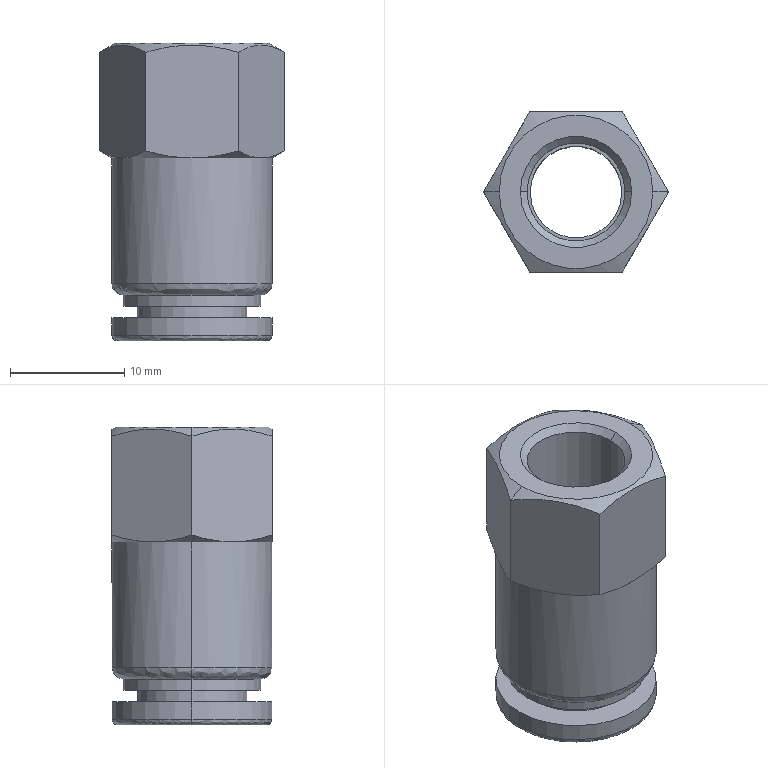Part | STEP file | APCF8-01 | 1 solid | 38 faces | box 16.166 x 14 x 26 mm | volume 2643 mm3 | cylinder 12 | cone 11 | plane 11 | spline 4 | commonest cylinder face diameters 14 x4 8 x2 8.566 x2 9.6 x2 12 x2
STEP:
#1=CARTESIAN_POINT('',(-7.,0.,5.));
#2=VERTEX_POINT('',#1);
#3=CARTESIAN_POINT('',(7.,0.,5.));
#4=VERTEX_POINT('',#3);
#5=CARTESIAN_POINT('',(0.,0.,5.));
#6=DIRECTION('',(0.,0.,1.));
#7=DIRECTION('',(-1.,0.,0.));
#8=AXIS2_PLACEMENT_3D('',#5,#6,#7);
#9=CIRCLE('',#8,7.);
#10=EDGE_CURVE('',#2,#4,#9,.T.);
#11=ORIENTED_EDGE('',*,*,#10,.F.);
#12=CARTESIAN_POINT('',(-6.,0.,4.));
#13=VERTEX_POINT('',#12);
#14=CARTESIAN_POINT('',(-6.,0.,5.));
#15=DIRECTION('',(0.,-1.,0.));
#16=DIRECTION('',(-1.,0.,0.));
#17=AXIS2_PLACEMENT_3D('',#14,#15,#16);
#18=CIRCLE('',#17,1.);
#19=EDGE_CURVE('',#2,#13,#18,.T.);
#20=ORIENTED_EDGE('',*,*,#19,.T.);
#21=CARTESIAN_POINT('',(6.,0.,4.));
#22=VERTEX_POINT('',#21);
#23=CARTESIAN_POINT('',(0.,0.,4.));
#24=DIRECTION('',(0.,0.,1.));
#25=DIRECTION('',(1.,0.,0.));
#26=AXIS2_PLACEMENT_3D('',#23,#24,#25);
#27=CIRCLE('',#26,6.);
#28=EDGE_CURVE('',#13,#22,#27,.T.);
#29=ORIENTED_EDGE('',*,*,#28,.T.);
#30=CARTESIAN_POINT('',(6.,0.,5.));
#31=DIRECTION('',(0.,1.,0.));
#32=DIRECTION('',(1.,0.,0.));
#33=AXIS2_PLACEMENT_3D('',#30,#31,#32);
#34=CIRCLE('',#33,1.);
#35=EDGE_CURVE('',#4,#22,#34,.T.);
#36=ORIENTED_EDGE('',*,*,#35,.F.);
#37=EDGE_LOOP('',(#11,#20,#29,#36));
#38=FACE_OUTER_BOUND('',#37,.T.);
#39=CARTESIAN_POINT('',(-7.,0.,5.));
#40=CARTESIAN_POINT('',(-7.,-14.,5.));
#41=CARTESIAN_POINT('',(7.,-14.,5.));
#42=CARTESIAN_POINT('',(7.,0.,5.));
#43=CARTESIAN_POINT('',(-7.,0.,4.414));
#44=CARTESIAN_POINT('',(-7.,-14.,4.414));
#45=CARTESIAN_POINT('',(7.,-14.,4.414));
#46=CARTESIAN_POINT('',(7.,0.,4.414));
#47=CARTESIAN_POINT('',(-6.586,0.,4.));
#48=CARTESIAN_POINT('',(-6.586,-13.172,4.));
#49=CARTESIAN_POINT('',(6.586,-13.172,4.));
#50=CARTESIAN_POINT('',(6.586,0.,4.));
#51=CARTESIAN_POINT('',(-6.,0.,4.));
#52=CARTESIAN_POINT('',(-6.,-12.,4.));
#53=CARTESIAN_POINT('',(6.,-12.,4.));
#54=CARTESIAN_POINT('',(6.,0.,4.));
#55=(BOUNDED_SURFACE()B_SPLINE_SURFACE(3,3,((#39,#40,#41,#42),(#43,#44,#45,#46),(#47,#48,#49,#50),(#51,#52,#53,#54)),.UNSPECIFIED.,.F.,.F.,.F.)B_SPLINE_SURFACE_WITH_KNOTS((4,4),(4,4),(0.,1.),(0.,1.),.UNSPECIFIED.)GEOMETRIC_REPRESENTATION_ITEM()RATIONAL_B_SPLINE_SURFACE(((1.,0.3333,0.3333,1.),(0.8047,0.2682,0.2682,0.8047),(0.8047,0.2682,0.2682,0.8047),(1.,0.3333,0.3333,1.)))REPRESENTATION_ITEM('')SURFACE());
#56=ADVANCED_FACE('',(#38),#55,.T.);
#57=CARTESIAN_POINT('',(-7.,0.,0.5));
#58=VERTEX_POINT('',#57);
#59=CARTESIAN_POINT('',(7.,0.,0.5));
#60=VERTEX_POINT('',#59);
#61=CARTESIAN_POINT('',(0.,0.,0.5));
#62=DIRECTION('',(0.,0.,1.));
#63=DIRECTION('',(-1.,0.,0.));
#64=AXIS2_PLACEMENT_3D('',#61,#62,#63);
#65=CIRCLE('',#64,7.);
#66=EDGE_CURVE('',#58,#60,#65,.T.);
#67=ORIENTED_EDGE('',*,*,#66,.F.);
#68=CARTESIAN_POINT('',(-6.5,0.,0.));
#69=VERTEX_POINT('',#68);
#70=CARTESIAN_POINT('',(-6.5,0.,0.5));
#71=DIRECTION('',(0.,-1.,0.));
#72=DIRECTION('',(-1.,0.,0.));
#73=AXIS2_PLACEMENT_3D('',#70,#71,#72);
#74=CIRCLE('',#73,0.5);
#75=EDGE_CURVE('',#58,#69,#74,.T.);
#76=ORIENTED_EDGE('',*,*,#75,.T.);
#77=CARTESIAN_POINT('',(6.5,0.,0.));
#78=VERTEX_POINT('',#77);
#79=CARTESIAN_POINT('',(-6.5,0.,0.));
#80=CARTESIAN_POINT('',(-6.5,-13.,0.));
#81=CARTESIAN_POINT('',(6.5,-13.,0.));
#82=CARTESIAN_POINT('',(6.5,0.,0.));
#83=(BOUNDED_CURVE()B_SPLINE_CURVE(3,(#79,#80,#81,#82),.UNSPECIFIED.,.F.,.T.)B_SPLINE_CURVE_WITH_KNOTS((4,4),(0.,1.),.UNSPECIFIED.)CURVE()GEOMETRIC_REPRESENTATION_ITEM()RATIONAL_B_SPLINE_CURVE((1.,0.3333,0.3333,1.))REPRESENTATION_ITEM(''));
#84=EDGE_CURVE('',#69,#78,#83,.T.);
#85=ORIENTED_EDGE('',*,*,#84,.T.);
#86=CARTESIAN_POINT('',(6.5,0.,0.5));
#87=DIRECTION('',(0.,1.,0.));
#88=DIRECTION('',(1.,0.,0.));
#89=AXIS2_PLACEMENT_3D('',#86,#87,#88);
#90=CIRCLE('',#89,0.5);
#91=EDGE_CURVE('',#60,#78,#90,.T.);
#92=ORIENTED_EDGE('',*,*,#91,.F.);
#93=EDGE_LOOP('',(#67,#76,#85,#92));
#94=FACE_OUTER_BOUND('',#93,.T.);
#95=CARTESIAN_POINT('',(-7.,0.,0.5));
#96=CARTESIAN_POINT('',(-7.,-14.,0.5));
#97=CARTESIAN_POINT('',(7.,-14.,0.5));
#98=CARTESIAN_POINT('',(7.,0.,0.5));
#99=CARTESIAN_POINT('',(-7.,0.,0.2071));
#100=CARTESIAN_POINT('',(-7.,-14.,0.2071));
#101=CARTESIAN_POINT('',(7.,-14.,0.2071));
#102=CARTESIAN_POINT('',(7.,0.,0.2071));
#103=CARTESIAN_POINT('',(-6.793,0.,0.));
#104=CARTESIAN_POINT('',(-6.793,-13.586,0.));
#105=CARTESIAN_POINT('',(6.793,-13.586,0.));
#106=CARTESIAN_POINT('',(6.793,0.,0.));
#107=CARTESIAN_POINT('',(-6.5,0.,0.));
#108=CARTESIAN_POINT('',(-6.5,-13.,0.));
#109=CARTESIAN_POINT('',(6.5,-13.,0.));
#110=CARTESIAN_POINT('',(6.5,0.,0.));
#111=(BOUNDED_SURFACE()B_SPLINE_SURFACE(3,3,((#95,#96,#97,#98),(#99,#100,#101,#102),(#103,#104,#105,#106),(#107,#108,#109,#110)),.UNSPECIFIED.,.F.,.F.,.F.)B_SPLINE_SURFACE_WITH_KNOTS((4,4),(4,4),(0.,1.),(0.,1.),.UNSPECIFIED.)GEOMETRIC_REPRESENTATION_ITEM()RATIONAL_B_SPLINE_SURFACE(((1.,0.3333,0.3333,1.),(0.8047,0.2682,0.2682,0.8047),(0.8047,0.2682,0.2682,0.8047),(1.,0.3333,0.3333,1.)))REPRESENTATION_ITEM('')SURFACE());
#112=ADVANCED_FACE('',(#94),#111,.T.);
#113=CARTESIAN_POINT('',(6.062,3.5,15.973));
#114=VERTEX_POINT('',#113);
#115=CARTESIAN_POINT('',(7.,0.,15.973));
#116=VERTEX_POINT('',#115);
#117=CARTESIAN_POINT('',(0.,0.,15.973));
#118=DIRECTION('',(0.,0.,-1.));
#119=DIRECTION('',(-1.,0.,0.));
#120=AXIS2_PLACEMENT_3D('',#117,#118,#119);
#121=CIRCLE('',#120,7.);
#122=EDGE_CURVE('',#114,#116,#121,.T.);
#123=ORIENTED_EDGE('',*,*,#122,.T.);
#124=CARTESIAN_POINT('',(7.,0.,10.487));
#125=DIRECTION('',(0.,0.,-1.));
#126=VECTOR('',#125,1000.);
#127=LINE('',#124,#126);
#128=EDGE_CURVE('',#116,#4,#127,.T.);
#129=ORIENTED_EDGE('',*,*,#128,.T.);
#130=CARTESIAN_POINT('',(0.,0.,5.));
#131=DIRECTION('',(0.,0.,1.));
#132=DIRECTION('',(-1.,0.,0.));
#133=AXIS2_PLACEMENT_3D('',#130,#131,#132);
#134=CIRCLE('',#133,7.);
#135=EDGE_CURVE('',#4,#2,#134,.T.);
#136=ORIENTED_EDGE('',*,*,#135,.T.);
#137=CARTESIAN_POINT('',(-7.,0.,15.973));
#138=VERTEX_POINT('',#137);
#139=CARTESIAN_POINT('',(-7.,0.,10.487));
#140=DIRECTION('',(0.,0.,-1.));
#141=VECTOR('',#140,1000.);
#142=LINE('',#139,#141);
#143=EDGE_CURVE('',#138,#2,#142,.T.);
#144=ORIENTED_EDGE('',*,*,#143,.F.);
#145=CARTESIAN_POINT('',(-6.062,3.5,15.973));
#146=VERTEX_POINT('',#145);
#147=CARTESIAN_POINT('',(0.,0.,15.973));
#148=DIRECTION('',(0.,0.,-1.));
#149=DIRECTION('',(-1.,0.,0.));
#150=AXIS2_PLACEMENT_3D('',#147,#148,#149);
#151=CIRCLE('',#150,7.);
#152=EDGE_CURVE('',#138,#146,#151,.T.);
#153=ORIENTED_EDGE('',*,*,#152,.T.);
#154=CARTESIAN_POINT('',(0.,7.,15.973));
#155=VERTEX_POINT('',#154);
#156=CARTESIAN_POINT('',(0.,0.,15.973));
#157=DIRECTION('',(0.,0.,-1.));
#158=DIRECTION('',(-1.,0.,0.));
#159=AXIS2_PLACEMENT_3D('',#156,#157,#158);
#160=CIRCLE('',#159,7.);
#161=EDGE_CURVE('',#146,#155,#160,.T.);
#162=ORIENTED_EDGE('',*,*,#161,.T.);
#163=CARTESIAN_POINT('',(0.,0.,15.973));
#164=DIRECTION('',(0.,0.,-1.));
#165=DIRECTION('',(-1.,0.,0.));
#166=AXIS2_PLACEMENT_3D('',#163,#164,#165);
#167=CIRCLE('',#166,7.);
#168=EDGE_CURVE('',#155,#114,#167,.T.);
#169=ORIENTED_EDGE('',*,*,#168,.T.);
#170=EDGE_LOOP('',(#123,#129,#136,#144,#153,#162,#169));
#171=FACE_OUTER_BOUND('',#170,.T.);
#172=CARTESIAN_POINT('',(0.,0.,10.487));
#173=DIRECTION('',(0.,0.,-1.));
#174=DIRECTION('',(-1.,0.,0.));
#175=AXIS2_PLACEMENT_3D('',#172,#173,#174);
#176=CYLINDRICAL_SURFACE('',#175,7.);
#177=ADVANCED_FACE('',(#171),#176,.T.);
#178=CARTESIAN_POINT('',(6.062,-3.5,15.973));
#179=VERTEX_POINT('',#178);
#180=CARTESIAN_POINT('',(0.,0.,15.973));
#181=DIRECTION('',(0.,0.,-1.));
#182=DIRECTION('',(-1.,0.,0.));
#183=AXIS2_PLACEMENT_3D('',#180,#181,#182);
#184=CIRCLE('',#183,7.);
#185=EDGE_CURVE('',#116,#179,#184,.T.);
#186=ORIENTED_EDGE('',*,*,#185,.F.);
#187=CARTESIAN_POINT('',(8.083,-0.000000012,16.598));
#188=VERTEX_POINT('',#187);
#189=CARTESIAN_POINT('',(8.089,0.,16.602));
#190=DIRECTION('',(0.866,0.,0.5));
#191=VECTOR('',#190,1000.);
#192=LINE('',#189,#191);
#193=EDGE_CURVE('',#116,#188,#192,.T.);
#194=ORIENTED_EDGE('',*,*,#193,.T.);
#195=CARTESIAN_POINT('',(8.083,-0.000000012,16.598));
#196=CARTESIAN_POINT('',(7.753,-0.5718,16.408));
#197=CARTESIAN_POINT('',(7.42,-1.148,16.251));
#198=CARTESIAN_POINT('',(6.747,-2.313,16.033));
#199=CARTESIAN_POINT('',(6.407,-2.903,15.973));
#200=CARTESIAN_POINT('',(6.062,-3.5,15.973));
#201=B_SPLINE_CURVE_WITH_KNOTS('',3,(#195,#196,#197,#198,#199,#200),.UNSPECIFIED.,.F.,.F.,(4,2,4),(0.,0.002045,0.00409),.UNSPECIFIED.);
#202=EDGE_CURVE('',#188,#179,#201,.T.);
#203=ORIENTED_EDGE('',*,*,#202,.T.);
#204=EDGE_LOOP('',(#186,#194,#203));
#205=FACE_OUTER_BOUND('',#204,.T.);
#206=CARTESIAN_POINT('',(0.,0.,16.602));
#207=DIRECTION('',(0.,0.,1.));
#208=DIRECTION('',(1.,0.,0.));
#209=AXIS2_PLACEMENT_3D('',#206,#207,#208);
#210=CONICAL_SURFACE('',#209,8.089,1.047);
#211=ADVANCED_FACE('',(#205),#210,.T.);
#212=CARTESIAN_POINT('',(0.,0.,4.));
#213=DIRECTION('',(0.,0.,1.));
#214=DIRECTION('',(1.,0.,0.));
#215=AXIS2_PLACEMENT_3D('',#212,#213,#214);
#216=CIRCLE('',#215,6.);
#217=EDGE_CURVE('',#22,#13,#216,.T.);
#218=ORIENTED_EDGE('',*,*,#217,.F.);
#219=CARTESIAN_POINT('',(6.,0.,3.));
#220=VERTEX_POINT('',#219);
#221=CARTESIAN_POINT('',(6.,0.,3.5));
#222=DIRECTION('',(0.,0.,-1.));
#223=VECTOR('',#222,1000.);
#224=LINE('',#221,#223);
#225=EDGE_CURVE('',#22,#220,#224,.T.);
#226=ORIENTED_EDGE('',*,*,#225,.T.);
#227=CARTESIAN_POINT('',(-6.,0.,3.));
#228=VERTEX_POINT('',#227);
#229=CARTESIAN_POINT('',(0.,0.,3.));
#230=DIRECTION('',(0.,0.,1.));
#231=DIRECTION('',(-1.,0.,0.));
#232=AXIS2_PLACEMENT_3D('',#229,#230,#231);
#233=CIRCLE('',#232,6.);
#234=EDGE_CURVE('',#220,#228,#233,.T.);
#235=ORIENTED_EDGE('',*,*,#234,.T.);
#236=CARTESIAN_POINT('',(-6.,0.,3.5));
#237=DIRECTION('',(0.,0.,-1.));
#238=VECTOR('',#237,1000.);
#239=LINE('',#236,#238);
#240=EDGE_CURVE('',#13,#228,#239,.T.);
#241=ORIENTED_EDGE('',*,*,#240,.F.);
#242=EDGE_LOOP('',(#218,#226,#235,#241));
#243=FACE_OUTER_BOUND('',#242,.T.);
#244=CARTESIAN_POINT('',(0.,0.,3.5));
#245=DIRECTION('',(0.,0.,-1.));
#246=DIRECTION('',(-1.,0.,0.));
#247=AXIS2_PLACEMENT_3D('',#244,#245,#246);
#248=CYLINDRICAL_SURFACE('',#247,6.);
#249=ADVANCED_FACE('',(#243),#248,.T.);
#250=CARTESIAN_POINT('',(-6.7,0.,26.));
#251=VERTEX_POINT('',#250);
#252=CARTESIAN_POINT('',(6.7,0.,26.));
#253=VERTEX_POINT('',#252);
#254=CARTESIAN_POINT('',(0.,0.,26.));
#255=DIRECTION('',(0.,0.,-1.));
#256=DIRECTION('',(-1.,0.,0.));
#257=AXIS2_PLACEMENT_3D('',#254,#255,#256);
#258=CIRCLE('',#257,6.7);
#259=EDGE_CURVE('',#251,#253,#258,.T.);
#260=ORIENTED_EDGE('',*,*,#259,.T.);
#261=CARTESIAN_POINT('',(8.083,0.,25.202));
#262=VERTEX_POINT('',#261);
#263=CARTESIAN_POINT('',(8.091,0.,25.197));
#264=DIRECTION('',(0.866,0.,-0.5));
#265=VECTOR('',#264,1000.);
#266=LINE('',#263,#265);
#267=EDGE_CURVE('',#253,#262,#266,.T.);
#268=ORIENTED_EDGE('',*,*,#267,.T.);
#269=CARTESIAN_POINT('',(4.041,7.,25.202));
#270=VERTEX_POINT('',#269);
#271=CARTESIAN_POINT('',(8.083,0.,25.202));
#272=CARTESIAN_POINT('',(7.753,0.5715,25.392));
#273=CARTESIAN_POINT('',(7.421,1.147,25.549));
#274=CARTESIAN_POINT('',(6.749,2.31,25.767));
#275=CARTESIAN_POINT('',(6.41,2.898,25.826));
#276=CARTESIAN_POINT('',(5.894,3.791,25.827));
#277=CARTESIAN_POINT('',(5.722,4.09,25.812));
#278=CARTESIAN_POINT('',(5.38,4.681,25.755));
#279=CARTESIAN_POINT('',(5.211,4.975,25.713));
#280=CARTESIAN_POINT('',(4.705,5.851,25.55));
#281=CARTESIAN_POINT('',(4.372,6.428,25.392));
#282=CARTESIAN_POINT('',(4.041,7.,25.202));
#283=B_SPLINE_CURVE_WITH_KNOTS('',3,(#271,#272,#273,#274,#275,#276,#277,#278,#279,#280,#281,#282),.UNSPECIFIED.,.F.,.F.,(4,2,2,2,2,4),(0.,0.002041,0.004082,0.005102,0.006122,0.008163),.UNSPECIFIED.);
#284=EDGE_CURVE('',#262,#270,#283,.T.);
#285=ORIENTED_EDGE('',*,*,#284,.T.);
#286=CARTESIAN_POINT('',(-4.041,7.,25.202));
#287=VERTEX_POINT('',#286);
#288=CARTESIAN_POINT('',(4.041,7.,25.202));
#289=CARTESIAN_POINT('',(3.381,7.,25.392));
#290=CARTESIAN_POINT('',(2.716,7.,25.549));
#291=CARTESIAN_POINT('',(1.37,7.,25.767));
#292=CARTESIAN_POINT('',(0.6897,7.,25.827));
#293=CARTESIAN_POINT('',(-0.6897,7.,25.827));
#294=CARTESIAN_POINT('',(-1.37,7.,25.767));
#295=CARTESIAN_POINT('',(-2.716,7.,25.549));
#296=CARTESIAN_POINT('',(-3.381,7.,25.392));
#297=CARTESIAN_POINT('',(-4.041,7.,25.202));
#298=B_SPLINE_CURVE_WITH_KNOTS('',3,(#288,#289,#290,#291,#292,#293,#294,#295,#296,#297),.UNSPECIFIED.,.F.,.F.,(4,2,2,2,4),(-0.00409,-0.002045,0.,0.002045,0.00409),.UNSPECIFIED.);
#299=EDGE_CURVE('',#270,#287,#298,.T.);
#300=ORIENTED_EDGE('',*,*,#299,.T.);
#301=CARTESIAN_POINT('',(-8.083,0.,25.202));
#302=VERTEX_POINT('',#301);
#303=CARTESIAN_POINT('',(-4.041,7.,25.202));
#304=CARTESIAN_POINT('',(-4.371,6.429,25.392));
#305=CARTESIAN_POINT('',(-4.704,5.853,25.549));
#306=CARTESIAN_POINT('',(-5.375,4.69,25.767));
#307=CARTESIAN_POINT('',(-5.715,4.102,25.826));
#308=CARTESIAN_POINT('',(-6.23,3.209,25.827));
#309=CARTESIAN_POINT('',(-6.403,2.91,25.812));
#310=CARTESIAN_POINT('',(-6.744,2.319,25.755));
#311=CARTESIAN_POINT('',(-6.914,2.025,25.713));
#312=CARTESIAN_POINT('',(-7.419,1.149,25.55));
#313=CARTESIAN_POINT('',(-7.753,0.5722,25.392));
#314=CARTESIAN_POINT('',(-8.083,0.,25.202));
#315=B_SPLINE_CURVE_WITH_KNOTS('',3,(#303,#304,#305,#306,#307,#308,#309,#310,#311,#312,#313,#314),.UNSPECIFIED.,.F.,.F.,(4,2,2,2,2,4),(0.,0.002041,0.004082,0.005102,0.006122,0.008163),.UNSPECIFIED.);
#316=EDGE_CURVE('',#287,#302,#315,.T.);
#317=ORIENTED_EDGE('',*,*,#316,.T.);
#318=CARTESIAN_POINT('',(-8.091,0.,25.197));
#319=DIRECTION('',(-0.866,0.,-0.5));
#320=VECTOR('',#319,1000.);
#321=LINE('',#318,#320);
#322=EDGE_CURVE('',#251,#302,#321,.T.);
#323=ORIENTED_EDGE('',*,*,#322,.F.);
#324=EDGE_LOOP('',(#260,#268,#285,#300,#317,#323));
#325=FACE_OUTER_BOUND('',#324,.T.);
#326=CARTESIAN_POINT('',(0.,0.,25.197));
#327=DIRECTION('',(0.,0.,-1.));
#328=DIRECTION('',(-1.,0.,0.));
#329=AXIS2_PLACEMENT_3D('',#326,#327,#328);
#330=CONICAL_SURFACE('',#329,8.091,1.047);
#331=ADVANCED_FACE('',(#325),#330,.T.);
#332=CARTESIAN_POINT('',(4.8,0.,3.));
#333=VERTEX_POINT('',#332);
#334=CARTESIAN_POINT('',(-4.8,0.,3.));
#335=VERTEX_POINT('',#334);
#336=CARTESIAN_POINT('',(0.,0.,3.));
#337=DIRECTION('',(0.,0.,1.));
#338=DIRECTION('',(-1.,0.,0.));
#339=AXIS2_PLACEMENT_3D('',#336,#337,#338);
#340=CIRCLE('',#339,4.8);
#341=EDGE_CURVE('',#333,#335,#340,.T.);
#342=ORIENTED_EDGE('',*,*,#341,.F.);
#343=CARTESIAN_POINT('',(4.8,0.,2.));
#344=VERTEX_POINT('',#343);
#345=CARTESIAN_POINT('',(4.8,0.,2.5));
#346=DIRECTION('',(0.,0.,-1.));
#347=VECTOR('',#346,1000.);
#348=LINE('',#345,#347);
#349=EDGE_CURVE('',#333,#344,#348,.T.);
#350=ORIENTED_EDGE('',*,*,#349,.T.);
#351=CARTESIAN_POINT('',(-4.8,0.,2.));
#352=VERTEX_POINT('',#351);
#353=CARTESIAN_POINT('',(0.,0.,2.));
#354=DIRECTION('',(0.,0.,1.));
#355=DIRECTION('',(-1.,0.,0.));
#356=AXIS2_PLACEMENT_3D('',#353,#354,#355);
#357=CIRCLE('',#356,4.8);
#358=EDGE_CURVE('',#344,#352,#357,.T.);
#359=ORIENTED_EDGE('',*,*,#358,.T.);
#360=CARTESIAN_POINT('',(-4.8,0.,2.5));
#361=DIRECTION('',(0.,0.,-1.));
#362=VECTOR('',#361,1000.);
#363=LINE('',#360,#362);
#364=EDGE_CURVE('',#335,#352,#363,.T.);
#365=ORIENTED_EDGE('',*,*,#364,.F.);
#366=EDGE_LOOP('',(#342,#350,#359,#365));
#367=FACE_OUTER_BOUND('',#366,.T.);
#368=CARTESIAN_POINT('',(0.,0.,2.5));
#369=DIRECTION('',(0.,0.,-1.));
#370=DIRECTION('',(-1.,0.,0.));
#371=AXIS2_PLACEMENT_3D('',#368,#369,#370);
#372=CYLINDRICAL_SURFACE('',#371,4.8);
#373=ADVANCED_FACE('',(#367),#372,.T.);
#374=CARTESIAN_POINT('',(-4.283,0.,25.419));
#375=VERTEX_POINT('',#374);
#376=CARTESIAN_POINT('',(4.283,0.,25.419));
#377=VERTEX_POINT('',#376);
#378=CARTESIAN_POINT('',(0.,0.,25.419));
#379=DIRECTION('',(0.,0.,1.));
#380=DIRECTION('',(0.,1.,0.));
#381=AXIS2_PLACEMENT_3D('',#378,#379,#380);
#382=CIRCLE('',#381,4.283);
#383=EDGE_CURVE('',#375,#377,#382,.T.);
#384=ORIENTED_EDGE('',*,*,#383,.F.);
#385=CARTESIAN_POINT('',(-4.864,0.,26.));
#386=VERTEX_POINT('',#385);
#387=CARTESIAN_POINT('',(-4.864,0.,26.));
#388=DIRECTION('',(-0.7071,0.,0.7071));
#389=VECTOR('',#388,1000.);
#390=LINE('',#387,#389);
#391=EDGE_CURVE('',#375,#386,#390,.T.);
#392=ORIENTED_EDGE('',*,*,#391,.T.);
#393=CARTESIAN_POINT('',(4.864,0.,26.));
#394=VERTEX_POINT('',#393);
#395=CARTESIAN_POINT('',(0.,0.,26.));
#396=DIRECTION('',(0.,0.,-1.));
#397=DIRECTION('',(1.,0.,0.));
#398=AXIS2_PLACEMENT_3D('',#395,#396,#397);
#399=CIRCLE('',#398,4.864);
#400=EDGE_CURVE('',#394,#386,#399,.T.);
#401=ORIENTED_EDGE('',*,*,#400,.F.);
#402=CARTESIAN_POINT('',(4.864,0.,26.));
#403=DIRECTION('',(0.7071,0.,0.7071));
#404=VECTOR('',#403,1000.);
#405=LINE('',#402,#404);
#406=EDGE_CURVE('',#377,#394,#405,.T.);
#407=ORIENTED_EDGE('',*,*,#406,.F.);
#408=EDGE_LOOP('',(#384,#392,#401,#407));
#409=FACE_OUTER_BOUND('',#408,.T.);
#410=CARTESIAN_POINT('',(0.,0.,26.));
#411=DIRECTION('',(0.,0.,1.));
#412=DIRECTION('',(1.,0.,0.));
#413=AXIS2_PLACEMENT_3D('',#410,#411,#412);
#414=CONICAL_SURFACE('',#413,4.864,0.7854);
#415=ADVANCED_FACE('',(#409),#414,.F.);
#416=CARTESIAN_POINT('',(7.,0.,2.));
#417=VERTEX_POINT('',#416);
#418=CARTESIAN_POINT('',(-7.,0.,2.));
#419=VERTEX_POINT('',#418);
#420=CARTESIAN_POINT('',(0.,0.,2.));
#421=DIRECTION('',(0.,0.,1.));
#422=DIRECTION('',(-1.,0.,0.));
#423=AXIS2_PLACEMENT_3D('',#420,#421,#422);
#424=CIRCLE('',#423,7.);
#425=EDGE_CURVE('',#417,#419,#424,.T.);
#426=ORIENTED_EDGE('',*,*,#425,.F.);
#427=CARTESIAN_POINT('',(7.,0.,1.25));
#428=DIRECTION('',(0.,0.,-1.));
#429=VECTOR('',#428,1000.);
#430=LINE('',#427,#429);
#431=EDGE_CURVE('',#417,#60,#430,.T.);
#432=ORIENTED_EDGE('',*,*,#431,.T.);
#433=CARTESIAN_POINT('',(0.,0.,0.5));
#434=DIRECTION('',(0.,0.,1.));
#435=DIRECTION('',(-1.,0.,0.));
#436=AXIS2_PLACEMENT_3D('',#433,#434,#435);
#437=CIRCLE('',#436,7.);
#438=EDGE_CURVE('',#60,#58,#437,.T.);
#439=ORIENTED_EDGE('',*,*,#438,.T.);
#440=CARTESIAN_POINT('',(-7.,0.,1.25));
#441=DIRECTION('',(0.,0.,-1.));
#442=VECTOR('',#441,1000.);
#443=LINE('',#440,#442);
#444=EDGE_CURVE('',#419,#58,#443,.T.);
#445=ORIENTED_EDGE('',*,*,#444,.F.);
#446=EDGE_LOOP('',(#426,#432,#439,#445));
#447=FACE_OUTER_BOUND('',#446,.T.);
#448=CARTESIAN_POINT('',(0.,0.,1.25));
#449=DIRECTION('',(0.,0.,-1.));
#450=DIRECTION('',(-1.,0.,0.));
#451=AXIS2_PLACEMENT_3D('',#448,#449,#450);
#452=CYLINDRICAL_SURFACE('',#451,7.);
#453=ADVANCED_FACE('',(#447),#452,.T.);
#454=ORIENTED_EDGE('',*,*,#383,.T.);
#455=CARTESIAN_POINT('',(4.283,0.,17.5));
#456=VERTEX_POINT('',#455);
#457=CARTESIAN_POINT('',(4.283,0.,21.459));
#458=DIRECTION('',(0.,0.,-1.));
#459=VECTOR('',#458,1000.);
#460=LINE('',#457,#459);
#461=EDGE_CURVE('',#377,#456,#460,.T.);
#462=ORIENTED_EDGE('',*,*,#461,.T.);
#463=CARTESIAN_POINT('',(-4.283,0.,17.5));
#464=VERTEX_POINT('',#463);
#465=CARTESIAN_POINT('',(0.,0.,17.5));
#466=DIRECTION('',(0.,0.,1.));
#467=DIRECTION('',(-1.,0.,0.));
#468=AXIS2_PLACEMENT_3D('',#465,#466,#467);
#469=CIRCLE('',#468,4.283);
#470=EDGE_CURVE('',#464,#456,#469,.T.);
#471=ORIENTED_EDGE('',*,*,#470,.F.);
#472=CARTESIAN_POINT('',(-4.283,0.,21.459));
#473=DIRECTION('',(0.,0.,-1.));
#474=VECTOR('',#473,1000.);
#475=LINE('',#472,#474);
#476=EDGE_CURVE('',#375,#464,#475,.T.);
#477=ORIENTED_EDGE('',*,*,#476,.F.);
#478=EDGE_LOOP('',(#454,#462,#471,#477));
#479=FACE_OUTER_BOUND('',#478,.T.);
#480=CARTESIAN_POINT('',(0.,0.,21.459));
#481=DIRECTION('',(0.,0.,-1.));
#482=DIRECTION('',(-1.,0.,0.));
#483=AXIS2_PLACEMENT_3D('',#480,#481,#482);
#484=CYLINDRICAL_SURFACE('',#483,4.283);
#485=ADVANCED_FACE('',(#479),#484,.F.);
#486=CARTESIAN_POINT('',(4.,0.,17.5));
#487=VERTEX_POINT('',#486);
#488=CARTESIAN_POINT('',(-4.,0.,17.5));
#489=VERTEX_POINT('',#488);
#490=CARTESIAN_POINT('',(0.,0.,17.5));
#491=DIRECTION('',(0.,0.,-1.));
#492=DIRECTION('',(-1.,0.,0.));
#493=AXIS2_PLACEMENT_3D('',#490,#491,#492);
#494=CIRCLE('',#493,4.);
#495=EDGE_CURVE('',#487,#489,#494,.T.);
#496=ORIENTED_EDGE('',*,*,#495,.F.);
#497=CARTESIAN_POINT('',(4.,0.,0.));
#498=VERTEX_POINT('',#497);
#499=CARTESIAN_POINT('',(4.,0.,8.75));
#500=DIRECTION('',(0.,0.,-1.));
#501=VECTOR('',#500,1000.);
#502=LINE('',#499,#501);
#503=EDGE_CURVE('',#487,#498,#502,.T.);
#504=ORIENTED_EDGE('',*,*,#503,.T.);
#505=CARTESIAN_POINT('',(-4.,0.,0.));
#506=VERTEX_POINT('',#505);
#507=CARTESIAN_POINT('',(0.,0.,0.));
#508=DIRECTION('',(0.,0.,1.));
#509=DIRECTION('',(-1.,0.,0.));
#510=AXIS2_PLACEMENT_3D('',#507,#508,#509);
#511=CIRCLE('',#510,4.);
#512=EDGE_CURVE('',#506,#498,#511,.T.);
#513=ORIENTED_EDGE('',*,*,#512,.F.);
#514=CARTESIAN_POINT('',(-4.,0.,8.75));
#515=DIRECTION('',(0.,0.,-1.));
#516=VECTOR('',#515,1000.);
#517=LINE('',#514,#516);
#518=EDGE_CURVE('',#489,#506,#517,.T.);
#519=ORIENTED_EDGE('',*,*,#518,.F.);
#520=EDGE_LOOP('',(#496,#504,#513,#519));
#521=FACE_OUTER_BOUND('',#520,.T.);
#522=CARTESIAN_POINT('',(0.,0.,8.75));
#523=DIRECTION('',(0.,0.,-1.));
#524=DIRECTION('',(-1.,0.,0.));
#525=AXIS2_PLACEMENT_3D('',#522,#523,#524);
#526=CYLINDRICAL_SURFACE('',#525,4.);
#527=ADVANCED_FACE('',(#521),#526,.F.);
#528=ORIENTED_EDGE('',*,*,#128,.F.);
#529=ORIENTED_EDGE('',*,*,#185,.T.);
#530=CARTESIAN_POINT('',(0.,-7.,15.973));
#531=VERTEX_POINT('',#530);
#532=CARTESIAN_POINT('',(0.,0.,15.973));
#533=DIRECTION('',(0.,0.,-1.));
#534=DIRECTION('',(-1.,0.,0.));
#535=AXIS2_PLACEMENT_3D('',#532,#533,#534);
#536=CIRCLE('',#535,7.);
#537=EDGE_CURVE('',#179,#531,#536,.T.);
#538=ORIENTED_EDGE('',*,*,#537,.T.);
#539=CARTESIAN_POINT('',(-6.062,-3.5,15.973));
#540=VERTEX_POINT('',#539);
#541=CARTESIAN_POINT('',(0.,0.,15.973));
#542=DIRECTION('',(0.,0.,-1.));
#543=DIRECTION('',(-1.,0.,0.));
#544=AXIS2_PLACEMENT_3D('',#541,#542,#543);
#545=CIRCLE('',#544,7.);
#546=EDGE_CURVE('',#531,#540,#545,.T.);
#547=ORIENTED_EDGE('',*,*,#546,.T.);
#548=CARTESIAN_POINT('',(0.,0.,15.973));
#549=DIRECTION('',(0.,0.,-1.));
#550=DIRECTION('',(-1.,0.,0.));
#551=AXIS2_PLACEMENT_3D('',#548,#549,#550);
#552=CIRCLE('',#551,7.);
#553=EDGE_CURVE('',#540,#138,#552,.T.);
#554=ORIENTED_EDGE('',*,*,#553,.T.);
#555=ORIENTED_EDGE('',*,*,#143,.T.);
#556=ORIENTED_EDGE('',*,*,#10,.T.);
#557=EDGE_LOOP('',(#528,#529,#538,#547,#554,#555,#556));
#558=FACE_OUTER_BOUND('',#557,.T.);
#559=CARTESIAN_POINT('',(0.,0.,10.487));
#560=DIRECTION('',(0.,0.,-1.));
#561=DIRECTION('',(-1.,0.,0.));
#562=AXIS2_PLACEMENT_3D('',#559,#560,#561);
#563=CYLINDRICAL_SURFACE('',#562,7.);
#564=ADVANCED_FACE('',(#558),#563,.T.);
#565=ORIENTED_EDGE('',*,*,#19,.F.);
#566=ORIENTED_EDGE('',*,*,#135,.F.);
#567=ORIENTED_EDGE('',*,*,#35,.T.);
#568=ORIENTED_EDGE('',*,*,#217,.T.);
#569=EDGE_LOOP('',(#565,#566,#567,#568));
#570=FACE_OUTER_BOUND('',#569,.T.);
#571=CARTESIAN_POINT('',(7.,0.,5.));
#572=CARTESIAN_POINT('',(7.,14.,5.));
#573=CARTESIAN_POINT('',(-7.,14.,5.));
#574=CARTESIAN_POINT('',(-7.,0.,5.));
#575=CARTESIAN_POINT('',(7.,0.,4.414));
#576=CARTESIAN_POINT('',(7.,14.,4.414));
#577=CARTESIAN_POINT('',(-7.,14.,4.414));
#578=CARTESIAN_POINT('',(-7.,0.,4.414));
#579=CARTESIAN_POINT('',(6.586,0.,4.));
#580=CARTESIAN_POINT('',(6.586,13.172,4.));
#581=CARTESIAN_POINT('',(-6.586,13.172,4.));
#582=CARTESIAN_POINT('',(-6.586,0.,4.));
#583=CARTESIAN_POINT('',(6.,0.,4.));
#584=CARTESIAN_POINT('',(6.,12.,4.));
#585=CARTESIAN_POINT('',(-6.,12.,4.));
#586=CARTESIAN_POINT('',(-6.,0.,4.));
#587=(BOUNDED_SURFACE()B_SPLINE_SURFACE(3,3,((#571,#572,#573,#574),(#575,#576,#577,#578),(#579,#580,#581,#582),(#583,#584,#585,#586)),.UNSPECIFIED.,.F.,.F.,.F.)B_SPLINE_SURFACE_WITH_KNOTS((4,4),(4,4),(0.,1.),(0.,1.),.UNSPECIFIED.)GEOMETRIC_REPRESENTATION_ITEM()RATIONAL_B_SPLINE_SURFACE(((1.,0.3333,0.3333,1.),(0.8047,0.2682,0.2682,0.8047),(0.8047,0.2682,0.2682,0.8047),(1.,0.3333,0.3333,1.)))REPRESENTATION_ITEM('')SURFACE());
#588=ADVANCED_FACE('',(#570),#587,.T.);
#589=CARTESIAN_POINT('',(4.041,-7.,16.598));
#590=VERTEX_POINT('',#589);
#591=CARTESIAN_POINT('',(4.041,-7.,16.598));
#592=CARTESIAN_POINT('',(3.381,-7.,16.408));
#593=CARTESIAN_POINT('',(2.716,-7.,16.251));
#594=CARTESIAN_POINT('',(1.37,-7.,16.033));
#595=CARTESIAN_POINT('',(0.6897,-7.,15.973));
#596=CARTESIAN_POINT('',(0.,-7.,15.973));
#597=B_SPLINE_CURVE_WITH_KNOTS('',3,(#591,#592,#593,#594,#595,#596),.UNSPECIFIED.,.F.,.F.,(4,2,4),(0.,0.002045,0.00409),.UNSPECIFIED.);
#598=EDGE_CURVE('',#590,#531,#597,.T.);
#599=ORIENTED_EDGE('',*,*,#598,.T.);
#600=ORIENTED_EDGE('',*,*,#537,.F.);
#601=CARTESIAN_POINT('',(6.062,-3.5,15.973));
#602=CARTESIAN_POINT('',(5.717,-4.097,15.973));
#603=CARTESIAN_POINT('',(5.377,-4.687,16.033));
#604=CARTESIAN_POINT('',(4.704,-5.852,16.251));
#605=CARTESIAN_POINT('',(4.372,-6.428,16.408));
#606=CARTESIAN_POINT('',(4.041,-7.,16.598));
#607=B_SPLINE_CURVE_WITH_KNOTS('',3,(#601,#602,#603,#604,#605,#606),.UNSPECIFIED.,.F.,.F.,(4,2,4),(0.,0.002045,0.00409),.UNSPECIFIED.);
#608=EDGE_CURVE('',#179,#590,#607,.T.);
#609=ORIENTED_EDGE('',*,*,#608,.T.);
#610=EDGE_LOOP('',(#599,#600,#609));
#611=FACE_OUTER_BOUND('',#610,.T.);
#612=CARTESIAN_POINT('',(0.,0.,16.602));
#613=DIRECTION('',(0.,0.,1.));
#614=DIRECTION('',(1.,0.,0.));
#615=AXIS2_PLACEMENT_3D('',#612,#613,#614);
#616=CONICAL_SURFACE('',#615,8.089,1.047);
#617=ADVANCED_FACE('',(#611),#616,.T.);
#618=ORIENTED_EDGE('',*,*,#193,.F.);
#619=ORIENTED_EDGE('',*,*,#122,.F.);
#620=CARTESIAN_POINT('',(6.062,3.5,15.973));
#621=CARTESIAN_POINT('',(6.407,2.903,15.973));
#622=CARTESIAN_POINT('',(6.747,2.313,16.033));
#623=CARTESIAN_POINT('',(7.42,1.148,16.251));
#624=CARTESIAN_POINT('',(7.753,0.5718,16.408));
#625=CARTESIAN_POINT('',(8.083,-0.000000012,16.598));
#626=B_SPLINE_CURVE_WITH_KNOTS('',3,(#620,#621,#622,#623,#624,#625),.UNSPECIFIED.,.F.,.F.,(4,2,4),(0.,0.002045,0.00409),.UNSPECIFIED.);
#627=EDGE_CURVE('',#114,#188,#626,.T.);
#628=ORIENTED_EDGE('',*,*,#627,.T.);
#629=EDGE_LOOP('',(#618,#619,#628));
#630=FACE_OUTER_BOUND('',#629,.T.);
#631=CARTESIAN_POINT('',(0.,0.,16.602));
#632=DIRECTION('',(0.,0.,1.));
#633=DIRECTION('',(1.,0.,0.));
#634=AXIS2_PLACEMENT_3D('',#631,#632,#633);
#635=CONICAL_SURFACE('',#634,8.089,1.047);
#636=ADVANCED_FACE('',(#630),#635,.T.);
#637=ORIENTED_EDGE('',*,*,#168,.F.);
#638=CARTESIAN_POINT('',(4.041,7.,16.598));
#639=VERTEX_POINT('',#638);
#640=CARTESIAN_POINT('',(0.,7.,15.973));
#641=CARTESIAN_POINT('',(0.6897,7.,15.973));
#642=CARTESIAN_POINT('',(1.37,7.,16.033));
#643=CARTESIAN_POINT('',(2.716,7.,16.251));
#644=CARTESIAN_POINT('',(3.381,7.,16.408));
#645=CARTESIAN_POINT('',(4.041,7.,16.598));
#646=B_SPLINE_CURVE_WITH_KNOTS('',3,(#640,#641,#642,#643,#644,#645),.UNSPECIFIED.,.F.,.F.,(4,2,4),(0.,0.002045,0.00409),.UNSPECIFIED.);
#647=EDGE_CURVE('',#155,#639,#646,.T.);
#648=ORIENTED_EDGE('',*,*,#647,.T.);
#649=CARTESIAN_POINT('',(4.041,7.,16.598));
#650=CARTESIAN_POINT('',(4.372,6.428,16.408));
#651=CARTESIAN_POINT('',(4.704,5.852,16.251));
#652=CARTESIAN_POINT('',(5.377,4.687,16.033));
#653=CARTESIAN_POINT('',(5.717,4.097,15.973));
#654=CARTESIAN_POINT('',(6.062,3.5,15.973));
#655=B_SPLINE_CURVE_WITH_KNOTS('',3,(#649,#650,#651,#652,#653,#654),.UNSPECIFIED.,.F.,.F.,(4,2,4),(0.,0.002045,0.00409),.UNSPECIFIED.);
#656=EDGE_CURVE('',#639,#114,#655,.T.);
#657=ORIENTED_EDGE('',*,*,#656,.T.);
#658=EDGE_LOOP('',(#637,#648,#657));
#659=FACE_OUTER_BOUND('',#658,.T.);
#660=CARTESIAN_POINT('',(0.,0.,16.602));
#661=DIRECTION('',(0.,0.,1.));
#662=DIRECTION('',(1.,0.,0.));
#663=AXIS2_PLACEMENT_3D('',#660,#661,#662);
#664=CONICAL_SURFACE('',#663,8.089,1.047);
#665=ADVANCED_FACE('',(#659),#664,.T.);
#666=ORIENTED_EDGE('',*,*,#225,.F.);
#667=ORIENTED_EDGE('',*,*,#28,.F.);
#668=ORIENTED_EDGE('',*,*,#240,.T.);
#669=CARTESIAN_POINT('',(0.,0.,3.));
#670=DIRECTION('',(0.,0.,1.));
#671=DIRECTION('',(-1.,0.,0.));
#672=AXIS2_PLACEMENT_3D('',#669,#670,#671);
#673=CIRCLE('',#672,6.);
#674=EDGE_CURVE('',#228,#220,#673,.T.);
#675=ORIENTED_EDGE('',*,*,#674,.T.);
#676=EDGE_LOOP('',(#666,#667,#668,#675));
#677=FACE_OUTER_BOUND('',#676,.T.);
#678=CARTESIAN_POINT('',(0.,0.,3.5));
#679=DIRECTION('',(0.,0.,-1.));
#680=DIRECTION('',(-1.,0.,0.));
#681=AXIS2_PLACEMENT_3D('',#678,#679,#680);
#682=CYLINDRICAL_SURFACE('',#681,6.);
#683=ADVANCED_FACE('',(#677),#682,.T.);
#684=ORIENTED_EDGE('',*,*,#161,.F.);
#685=CARTESIAN_POINT('',(-4.041,7.,16.598));
#686=VERTEX_POINT('',#685);
#687=CARTESIAN_POINT('',(-6.062,3.5,15.973));
#688=CARTESIAN_POINT('',(-5.717,4.097,15.973));
#689=CARTESIAN_POINT('',(-5.377,4.687,16.033));
#690=CARTESIAN_POINT('',(-4.704,5.852,16.251));
#691=CARTESIAN_POINT('',(-4.372,6.428,16.408));
#692=CARTESIAN_POINT('',(-4.041,7.,16.598));
#693=B_SPLINE_CURVE_WITH_KNOTS('',3,(#687,#688,#689,#690,#691,#692),.UNSPECIFIED.,.F.,.F.,(4,2,4),(0.,0.002045,0.00409),.UNSPECIFIED.);
#694=EDGE_CURVE('',#146,#686,#693,.T.);
#695=ORIENTED_EDGE('',*,*,#694,.T.);
#696=CARTESIAN_POINT('',(-4.041,7.,16.598));
#697=CARTESIAN_POINT('',(-3.381,7.,16.408));
#698=CARTESIAN_POINT('',(-2.716,7.,16.251));
#699=CARTESIAN_POINT('',(-1.37,7.,16.033));
#700=CARTESIAN_POINT('',(-0.6897,7.,15.973));
#701=CARTESIAN_POINT('',(0.,7.,15.973));
#702=B_SPLINE_CURVE_WITH_KNOTS('',3,(#696,#697,#698,#699,#700,#701),.UNSPECIFIED.,.F.,.F.,(4,2,4),(0.,0.002045,0.00409),.UNSPECIFIED.);
#703=EDGE_CURVE('',#686,#155,#702,.T.);
#704=ORIENTED_EDGE('',*,*,#703,.T.);
#705=EDGE_LOOP('',(#684,#695,#704));
#706=FACE_OUTER_BOUND('',#705,.T.);
#707=CARTESIAN_POINT('',(0.,0.,16.602));
#708=DIRECTION('',(0.,0.,1.));
#709=DIRECTION('',(1.,0.,0.));
#710=AXIS2_PLACEMENT_3D('',#707,#708,#709);
#711=CONICAL_SURFACE('',#710,8.089,1.047);
#712=ADVANCED_FACE('',(#706),#711,.T.);
#713=ORIENTED_EDGE('',*,*,#553,.F.);
#714=CARTESIAN_POINT('',(-8.083,0.000000038,16.598));
#715=VERTEX_POINT('',#714);
#716=CARTESIAN_POINT('',(-6.062,-3.5,15.973));
#717=CARTESIAN_POINT('',(-6.407,-2.903,15.973));
#718=CARTESIAN_POINT('',(-6.747,-2.313,16.033));
#719=CARTESIAN_POINT('',(-7.42,-1.148,16.251));
#720=CARTESIAN_POINT('',(-7.753,-0.5718,16.408));
#721=CARTESIAN_POINT('',(-8.083,0.000000038,16.598));
#722=B_SPLINE_CURVE_WITH_KNOTS('',3,(#716,#717,#718,#719,#720,#721),.UNSPECIFIED.,.F.,.F.,(4,2,4),(0.,0.002045,0.00409),.UNSPECIFIED.);
#723=EDGE_CURVE('',#540,#715,#722,.T.);
#724=ORIENTED_EDGE('',*,*,#723,.T.);
#725=CARTESIAN_POINT('',(-8.083,0.000000038,16.598));
#726=CARTESIAN_POINT('',(-7.753,0.5718,16.408));
#727=CARTESIAN_POINT('',(-7.42,1.148,16.251));
#728=CARTESIAN_POINT('',(-6.747,2.313,16.033));
#729=CARTESIAN_POINT('',(-6.407,2.903,15.973));
#730=CARTESIAN_POINT('',(-6.062,3.5,15.973));
#731=B_SPLINE_CURVE_WITH_KNOTS('',3,(#725,#726,#727,#728,#729,#730),.UNSPECIFIED.,.F.,.F.,(4,2,4),(0.,0.002045,0.00409),.UNSPECIFIED.);
#732=EDGE_CURVE('',#715,#146,#731,.T.);
#733=ORIENTED_EDGE('',*,*,#732,.T.);
#734=ORIENTED_EDGE('',*,*,#152,.F.);
#735=EDGE_LOOP('',(#713,#724,#733,#734));
#736=FACE_OUTER_BOUND('',#735,.T.);
#737=CARTESIAN_POINT('',(0.,0.,16.602));
#738=DIRECTION('',(0.,0.,1.));
#739=DIRECTION('',(1.,0.,0.));
#740=AXIS2_PLACEMENT_3D('',#737,#738,#739);
#741=CONICAL_SURFACE('',#740,8.089,1.047);
#742=ADVANCED_FACE('',(#736),#741,.T.);
#743=CARTESIAN_POINT('',(-4.041,-7.,16.598));
#744=VERTEX_POINT('',#743);
#745=CARTESIAN_POINT('',(-4.041,-7.,16.598));
#746=CARTESIAN_POINT('',(-4.372,-6.428,16.408));
#747=CARTESIAN_POINT('',(-4.704,-5.852,16.251));
#748=CARTESIAN_POINT('',(-5.377,-4.687,16.033));
#749=CARTESIAN_POINT('',(-5.717,-4.097,15.973));
#750=CARTESIAN_POINT('',(-6.062,-3.5,15.973));
#751=B_SPLINE_CURVE_WITH_KNOTS('',3,(#745,#746,#747,#748,#749,#750),.UNSPECIFIED.,.F.,.F.,(4,2,4),(0.,0.002045,0.00409),.UNSPECIFIED.);
#752=EDGE_CURVE('',#744,#540,#751,.T.);
#753=ORIENTED_EDGE('',*,*,#752,.T.);
#754=ORIENTED_EDGE('',*,*,#546,.F.);
#755=CARTESIAN_POINT('',(0.,-7.,15.973));
#756=CARTESIAN_POINT('',(-0.6897,-7.,15.973));
#757=CARTESIAN_POINT('',(-1.37,-7.,16.033));
#758=CARTESIAN_POINT('',(-2.716,-7.,16.251));
#759=CARTESIAN_POINT('',(-3.381,-7.,16.408));
#760=CARTESIAN_POINT('',(-4.041,-7.,16.598));
#761=B_SPLINE_CURVE_WITH_KNOTS('',3,(#755,#756,#757,#758,#759,#760),.UNSPECIFIED.,.F.,.F.,(4,2,4),(0.,0.002045,0.00409),.UNSPECIFIED.);
#762=EDGE_CURVE('',#531,#744,#761,.T.);
#763=ORIENTED_EDGE('',*,*,#762,.T.);
#764=EDGE_LOOP('',(#753,#754,#763));
#765=FACE_OUTER_BOUND('',#764,.T.);
#766=CARTESIAN_POINT('',(0.,0.,16.602));
#767=DIRECTION('',(0.,0.,1.));
#768=DIRECTION('',(1.,0.,0.));
#769=AXIS2_PLACEMENT_3D('',#766,#767,#768);
#770=CONICAL_SURFACE('',#769,8.089,1.047);
#771=ADVANCED_FACE('',(#765),#770,.T.);
#772=CARTESIAN_POINT('',(-4.041,-7.,25.202));
#773=VERTEX_POINT('',#772);
#774=CARTESIAN_POINT('',(-4.041,-7.,26.));
#775=DIRECTION('',(0.,0.,1.));
#776=VECTOR('',#775,1000.);
#777=LINE('',#774,#776);
#778=EDGE_CURVE('',#744,#773,#777,.T.);
#779=ORIENTED_EDGE('',*,*,#778,.F.);
#780=ORIENTED_EDGE('',*,*,#762,.F.);
#781=ORIENTED_EDGE('',*,*,#598,.F.);
#782=CARTESIAN_POINT('',(4.041,-7.,25.202));
#783=VERTEX_POINT('',#782);
#784=CARTESIAN_POINT('',(4.041,-7.,26.));
#785=DIRECTION('',(0.,0.,-1.));
#786=VECTOR('',#785,1000.);
#787=LINE('',#784,#786);
#788=EDGE_CURVE('',#783,#590,#787,.T.);
#789=ORIENTED_EDGE('',*,*,#788,.F.);
#790=CARTESIAN_POINT('',(-4.041,-7.,25.202));
#791=CARTESIAN_POINT('',(-3.381,-7.,25.392));
#792=CARTESIAN_POINT('',(-2.716,-7.,25.549));
#793=CARTESIAN_POINT('',(-1.37,-7.,25.767));
#794=CARTESIAN_POINT('',(-0.6897,-7.,25.827));
#795=CARTESIAN_POINT('',(0.6897,-7.,25.827));
#796=CARTESIAN_POINT('',(1.37,-7.,25.767));
#797=CARTESIAN_POINT('',(2.716,-7.,25.549));
#798=CARTESIAN_POINT('',(3.381,-7.,25.392));
#799=CARTESIAN_POINT('',(4.041,-7.,25.202));
#800=B_SPLINE_CURVE_WITH_KNOTS('',3,(#790,#791,#792,#793,#794,#795,#796,#797,#798,#799),.UNSPECIFIED.,.F.,.F.,(4,2,2,2,4),(0.,0.002045,0.00409,0.006134,0.008179),.UNSPECIFIED.);
#801=EDGE_CURVE('',#773,#783,#800,.T.);
#802=ORIENTED_EDGE('',*,*,#801,.F.);
#803=EDGE_LOOP('',(#779,#780,#781,#789,#802));
#804=FACE_OUTER_BOUND('',#803,.T.);
#805=CARTESIAN_POINT('',(4.041,-7.,26.));
#806=DIRECTION('',(0.,1.,0.));
#807=DIRECTION('',(0.,0.,1.));
#808=AXIS2_PLACEMENT_3D('',#805,#806,#807);
#809=PLANE('',#808);
#810=ADVANCED_FACE('',(#804),#809,.F.);
#811=CARTESIAN_POINT('',(8.083,0.,26.));
#812=DIRECTION('',(0.,0.,-1.));
#813=VECTOR('',#812,1000.);
#814=LINE('',#811,#813);
#815=EDGE_CURVE('',#262,#188,#814,.T.);
#816=ORIENTED_EDGE('',*,*,#815,.F.);
#817=CARTESIAN_POINT('',(4.041,-7.,25.202));
#818=CARTESIAN_POINT('',(4.371,-6.429,25.392));
#819=CARTESIAN_POINT('',(4.704,-5.853,25.549));
#820=CARTESIAN_POINT('',(5.375,-4.69,25.767));
#821=CARTESIAN_POINT('',(5.715,-4.102,25.826));
#822=CARTESIAN_POINT('',(6.23,-3.209,25.827));
#823=CARTESIAN_POINT('',(6.403,-2.91,25.812));
#824=CARTESIAN_POINT('',(6.744,-2.319,25.755));
#825=CARTESIAN_POINT('',(6.914,-2.025,25.713));
#826=CARTESIAN_POINT('',(7.419,-1.149,25.55));
#827=CARTESIAN_POINT('',(7.753,-0.5722,25.392));
#828=CARTESIAN_POINT('',(8.083,0.,25.202));
#829=B_SPLINE_CURVE_WITH_KNOTS('',3,(#817,#818,#819,#820,#821,#822,#823,#824,#825,#826,#827,#828),.UNSPECIFIED.,.F.,.F.,(4,2,2,2,2,4),(0.,0.002041,0.004082,0.005102,0.006122,0.008163),.UNSPECIFIED.);
#830=EDGE_CURVE('',#783,#262,#829,.T.);
#831=ORIENTED_EDGE('',*,*,#830,.F.);
#832=ORIENTED_EDGE('',*,*,#788,.T.);
#833=ORIENTED_EDGE('',*,*,#608,.F.);
#834=ORIENTED_EDGE('',*,*,#202,.F.);
#835=EDGE_LOOP('',(#816,#831,#832,#833,#834));
#836=FACE_OUTER_BOUND('',#835,.T.);
#837=CARTESIAN_POINT('',(8.083,0.,26.));
#838=DIRECTION('',(-0.866,0.5,0.));
#839=DIRECTION('',(-0.5,-0.866,0.));
#840=AXIS2_PLACEMENT_3D('',#837,#838,#839);
#841=PLANE('',#840);
#842=ADVANCED_FACE('',(#836),#841,.F.);
#843=ORIENTED_EDGE('',*,*,#656,.F.);
#844=CARTESIAN_POINT('',(4.041,7.,26.));
#845=DIRECTION('',(0.,0.,-1.));
#846=VECTOR('',#845,1000.);
#847=LINE('',#844,#846);
#848=EDGE_CURVE('',#270,#639,#847,.T.);
#849=ORIENTED_EDGE('',*,*,#848,.F.);
#850=ORIENTED_EDGE('',*,*,#284,.F.);
#851=ORIENTED_EDGE('',*,*,#815,.T.);
#852=ORIENTED_EDGE('',*,*,#627,.F.);
#853=EDGE_LOOP('',(#843,#849,#850,#851,#852));
#854=FACE_OUTER_BOUND('',#853,.T.);
#855=CARTESIAN_POINT('',(4.041,7.,26.));
#856=DIRECTION('',(-0.866,-0.5,0.));
#857=DIRECTION('',(0.5,-0.866,0.));
#858=AXIS2_PLACEMENT_3D('',#855,#856,#857);
#859=PLANE('',#858);
#860=ADVANCED_FACE('',(#854),#859,.F.);
#861=ORIENTED_EDGE('',*,*,#703,.F.);
#862=CARTESIAN_POINT('',(-4.041,7.,26.));
#863=DIRECTION('',(0.,0.,-1.));
#864=VECTOR('',#863,1000.);
#865=LINE('',#862,#864);
#866=EDGE_CURVE('',#287,#686,#865,.T.);
#867=ORIENTED_EDGE('',*,*,#866,.F.);
#868=ORIENTED_EDGE('',*,*,#299,.F.);
#869=ORIENTED_EDGE('',*,*,#848,.T.);
#870=ORIENTED_EDGE('',*,*,#647,.F.);
#871=EDGE_LOOP('',(#861,#867,#868,#869,#870));
#872=FACE_OUTER_BOUND('',#871,.T.);
#873=CARTESIAN_POINT('',(-4.041,7.,26.));
#874=DIRECTION('',(0.,-1.,0.));
#875=DIRECTION('',(0.,0.,-1.));
#876=AXIS2_PLACEMENT_3D('',#873,#874,#875);
#877=PLANE('',#876);
#878=ADVANCED_FACE('',(#872),#877,.F.);
#879=CARTESIAN_POINT('',(0.,0.,3.));
#880=DIRECTION('',(0.,0.,1.));
#881=DIRECTION('',(-1.,0.,0.));
#882=AXIS2_PLACEMENT_3D('',#879,#880,#881);
#883=CIRCLE('',#882,4.8);
#884=EDGE_CURVE('',#335,#333,#883,.T.);
#885=ORIENTED_EDGE('',*,*,#884,.T.);
#886=ORIENTED_EDGE('',*,*,#341,.T.);
#887=EDGE_LOOP('',(#885,#886));
#888=FACE_BOUND('',#887,.T.);
#889=ORIENTED_EDGE('',*,*,#674,.F.);
#890=ORIENTED_EDGE('',*,*,#234,.F.);
#891=EDGE_LOOP('',(#889,#890));
#892=FACE_OUTER_BOUND('',#891,.T.);
#893=CARTESIAN_POINT('',(0.,5.4,3.));
#894=DIRECTION('',(0.,0.,-1.));
#895=DIRECTION('',(-1.,0.,0.));
#896=AXIS2_PLACEMENT_3D('',#893,#894,#895);
#897=PLANE('',#896);
#898=ADVANCED_FACE('',(#888,#892),#897,.T.);
#899=ORIENTED_EDGE('',*,*,#732,.F.);
#900=CARTESIAN_POINT('',(-8.083,0.,26.));
#901=DIRECTION('',(0.,0.,-1.));
#902=VECTOR('',#901,1000.);
#903=LINE('',#900,#902);
#904=EDGE_CURVE('',#302,#715,#903,.T.);
#905=ORIENTED_EDGE('',*,*,#904,.F.);
#906=ORIENTED_EDGE('',*,*,#316,.F.);
#907=ORIENTED_EDGE('',*,*,#866,.T.);
#908=ORIENTED_EDGE('',*,*,#694,.F.);
#909=EDGE_LOOP('',(#899,#905,#906,#907,#908));
#910=FACE_OUTER_BOUND('',#909,.T.);
#911=CARTESIAN_POINT('',(-8.083,0.,26.));
#912=DIRECTION('',(0.866,-0.5,0.));
#913=DIRECTION('',(0.5,0.866,0.));
#914=AXIS2_PLACEMENT_3D('',#911,#912,#913);
#915=PLANE('',#914);
#916=ADVANCED_FACE('',(#910),#915,.F.);
#917=ORIENTED_EDGE('',*,*,#904,.T.);
#918=ORIENTED_EDGE('',*,*,#723,.F.);
#919=ORIENTED_EDGE('',*,*,#752,.F.);
#920=ORIENTED_EDGE('',*,*,#778,.T.);
#921=CARTESIAN_POINT('',(-8.083,0.,25.202));
#922=CARTESIAN_POINT('',(-7.753,-0.5715,25.392));
#923=CARTESIAN_POINT('',(-7.421,-1.147,25.549));
#924=CARTESIAN_POINT('',(-6.749,-2.31,25.767));
#925=CARTESIAN_POINT('',(-6.41,-2.898,25.826));
#926=CARTESIAN_POINT('',(-5.894,-3.791,25.827));
#927=CARTESIAN_POINT('',(-5.722,-4.09,25.812));
#928=CARTESIAN_POINT('',(-5.38,-4.681,25.755));
#929=CARTESIAN_POINT('',(-5.211,-4.975,25.713));
#930=CARTESIAN_POINT('',(-4.705,-5.851,25.55));
#931=CARTESIAN_POINT('',(-4.372,-6.428,25.392));
#932=CARTESIAN_POINT('',(-4.041,-7.,25.202));
#933=B_SPLINE_CURVE_WITH_KNOTS('',3,(#921,#922,#923,#924,#925,#926,#927,#928,#929,#930,#931,#932),.UNSPECIFIED.,.F.,.F.,(4,2,2,2,2,4),(0.,0.002041,0.004082,0.005102,0.006122,0.008163),.UNSPECIFIED.);
#934=EDGE_CURVE('',#302,#773,#933,.T.);
#935=ORIENTED_EDGE('',*,*,#934,.F.);
#936=EDGE_LOOP('',(#917,#918,#919,#920,#935));
#937=FACE_OUTER_BOUND('',#936,.T.);
#938=CARTESIAN_POINT('',(-4.041,-7.,26.));
#939=DIRECTION('',(0.866,0.5,0.));
#940=DIRECTION('',(-0.5,0.866,0.));
#941=AXIS2_PLACEMENT_3D('',#938,#939,#940);
#942=PLANE('',#941);
#943=ADVANCED_FACE('',(#937),#942,.F.);
#944=ORIENTED_EDGE('',*,*,#267,.F.);
#945=CARTESIAN_POINT('',(0.,0.,26.));
#946=DIRECTION('',(0.,0.,-1.));
#947=DIRECTION('',(-1.,0.,0.));
#948=AXIS2_PLACEMENT_3D('',#945,#946,#947);
#949=CIRCLE('',#948,6.7);
#950=EDGE_CURVE('',#253,#251,#949,.T.);
#951=ORIENTED_EDGE('',*,*,#950,.T.);
#952=ORIENTED_EDGE('',*,*,#322,.T.);
#953=ORIENTED_EDGE('',*,*,#934,.T.);
#954=ORIENTED_EDGE('',*,*,#801,.T.);
#955=ORIENTED_EDGE('',*,*,#830,.T.);
#956=EDGE_LOOP('',(#944,#951,#952,#953,#954,#955));
#957=FACE_OUTER_BOUND('',#956,.T.);
#958=CARTESIAN_POINT('',(0.,0.,25.197));
#959=DIRECTION('',(0.,0.,-1.));
#960=DIRECTION('',(-1.,0.,0.));
#961=AXIS2_PLACEMENT_3D('',#958,#959,#960);
#962=CONICAL_SURFACE('',#961,8.091,1.047);
#963=ADVANCED_FACE('',(#957),#962,.T.);
#964=ORIENTED_EDGE('',*,*,#349,.F.);
#965=ORIENTED_EDGE('',*,*,#884,.F.);
#966=ORIENTED_EDGE('',*,*,#364,.T.);
#967=CARTESIAN_POINT('',(0.,0.,2.));
#968=DIRECTION('',(0.,0.,1.));
#969=DIRECTION('',(-1.,0.,0.));
#970=AXIS2_PLACEMENT_3D('',#967,#968,#969);
#971=CIRCLE('',#970,4.8);
#972=EDGE_CURVE('',#352,#344,#971,.T.);
#973=ORIENTED_EDGE('',*,*,#972,.T.);
#974=EDGE_LOOP('',(#964,#965,#966,#973));
#975=FACE_OUTER_BOUND('',#974,.T.);
#976=CARTESIAN_POINT('',(0.,0.,2.5));
#977=DIRECTION('',(0.,0.,-1.));
#978=DIRECTION('',(-1.,0.,0.));
#979=AXIS2_PLACEMENT_3D('',#976,#977,#978);
#980=CYLINDRICAL_SURFACE('',#979,4.8);
#981=ADVANCED_FACE('',(#975),#980,.T.);
#982=ORIENTED_EDGE('',*,*,#259,.F.);
#983=ORIENTED_EDGE('',*,*,#950,.F.);
#984=EDGE_LOOP('',(#982,#983));
#985=FACE_OUTER_BOUND('',#984,.T.);
#986=ORIENTED_EDGE('',*,*,#400,.T.);
#987=CARTESIAN_POINT('',(0.,0.,26.));
#988=DIRECTION('',(0.,0.,-1.));
#989=DIRECTION('',(1.,0.,0.));
#990=AXIS2_PLACEMENT_3D('',#987,#988,#989);
#991=CIRCLE('',#990,4.864);
#992=EDGE_CURVE('',#386,#394,#991,.T.);
#993=ORIENTED_EDGE('',*,*,#992,.T.);
#994=EDGE_LOOP('',(#986,#993));
#995=FACE_BOUND('',#994,.T.);
#996=CARTESIAN_POINT('',(0.,5.782,26.));
#997=DIRECTION('',(0.,0.,1.));
#998=DIRECTION('',(1.,0.,0.));
#999=AXIS2_PLACEMENT_3D('',#996,#997,#998);
#1000=PLANE('',#999);
#1001=ADVANCED_FACE('',(#985,#995),#1000,.T.);
#1002=CARTESIAN_POINT('',(0.,0.,2.));
#1003=DIRECTION('',(0.,0.,1.));
#1004=DIRECTION('',(-1.,0.,0.));
#1005=AXIS2_PLACEMENT_3D('',#1002,#1003,#1004);
#1006=CIRCLE('',#1005,7.);
#1007=EDGE_CURVE('',#419,#417,#1006,.T.);
#1008=ORIENTED_EDGE('',*,*,#1007,.T.);
#1009=ORIENTED_EDGE('',*,*,#425,.T.);
#1010=EDGE_LOOP('',(#1008,#1009));
#1011=FACE_OUTER_BOUND('',#1010,.T.);
#1012=ORIENTED_EDGE('',*,*,#972,.F.);
#1013=ORIENTED_EDGE('',*,*,#358,.F.);
#1014=EDGE_LOOP('',(#1012,#1013));
#1015=FACE_BOUND('',#1014,.T.);
#1016=CARTESIAN_POINT('',(0.,5.9,2.));
#1017=DIRECTION('',(0.,0.,1.));
#1018=DIRECTION('',(1.,0.,0.));
#1019=AXIS2_PLACEMENT_3D('',#1016,#1017,#1018);
#1020=PLANE('',#1019);
#1021=ADVANCED_FACE('',(#1011,#1015),#1020,.T.);
#1022=ORIENTED_EDGE('',*,*,#391,.F.);
#1023=CARTESIAN_POINT('',(0.,0.,25.419));
#1024=DIRECTION('',(0.,0.,1.));
#1025=DIRECTION('',(0.,1.,0.));
#1026=AXIS2_PLACEMENT_3D('',#1023,#1024,#1025);
#1027=CIRCLE('',#1026,4.283);
#1028=EDGE_CURVE('',#377,#375,#1027,.T.);
#1029=ORIENTED_EDGE('',*,*,#1028,.F.);
#1030=ORIENTED_EDGE('',*,*,#406,.T.);
#1031=ORIENTED_EDGE('',*,*,#992,.F.);
#1032=EDGE_LOOP('',(#1022,#1029,#1030,#1031));
#1033=FACE_OUTER_BOUND('',#1032,.T.);
#1034=CARTESIAN_POINT('',(0.,0.,26.));
#1035=DIRECTION('',(0.,0.,1.));
#1036=DIRECTION('',(1.,0.,0.));
#1037=AXIS2_PLACEMENT_3D('',#1034,#1035,#1036);
#1038=CONICAL_SURFACE('',#1037,4.864,0.7854);
#1039=ADVANCED_FACE('',(#1033),#1038,.F.);
#1040=ORIENTED_EDGE('',*,*,#431,.F.);
#1041=ORIENTED_EDGE('',*,*,#1007,.F.);
#1042=ORIENTED_EDGE('',*,*,#444,.T.);
#1043=ORIENTED_EDGE('',*,*,#66,.T.);
#1044=EDGE_LOOP('',(#1040,#1041,#1042,#1043));
#1045=FACE_OUTER_BOUND('',#1044,.T.);
#1046=CARTESIAN_POINT('',(0.,0.,1.25));
#1047=DIRECTION('',(0.,0.,-1.));
#1048=DIRECTION('',(-1.,0.,0.));
#1049=AXIS2_PLACEMENT_3D('',#1046,#1047,#1048);
#1050=CYLINDRICAL_SURFACE('',#1049,7.);
#1051=ADVANCED_FACE('',(#1045),#1050,.T.);
#1052=ORIENTED_EDGE('',*,*,#461,.F.);
#1053=ORIENTED_EDGE('',*,*,#1028,.T.);
#1054=ORIENTED_EDGE('',*,*,#476,.T.);
#1055=CARTESIAN_POINT('',(0.,0.,17.5));
#1056=DIRECTION('',(0.,0.,1.));
#1057=DIRECTION('',(-1.,0.,0.));
#1058=AXIS2_PLACEMENT_3D('',#1055,#1056,#1057);
#1059=CIRCLE('',#1058,4.283);
#1060=EDGE_CURVE('',#456,#464,#1059,.T.);
#1061=ORIENTED_EDGE('',*,*,#1060,.F.);
#1062=EDGE_LOOP('',(#1052,#1053,#1054,#1061));
#1063=FACE_OUTER_BOUND('',#1062,.T.);
#1064=CARTESIAN_POINT('',(0.,0.,21.459));
#1065=DIRECTION('',(0.,0.,-1.));
#1066=DIRECTION('',(-1.,0.,0.));
#1067=AXIS2_PLACEMENT_3D('',#1064,#1065,#1066);
#1068=CYLINDRICAL_SURFACE('',#1067,4.283);
#1069=ADVANCED_FACE('',(#1063),#1068,.F.);
#1070=ORIENTED_EDGE('',*,*,#75,.F.);
#1071=ORIENTED_EDGE('',*,*,#438,.F.);
#1072=ORIENTED_EDGE('',*,*,#91,.T.);
#1073=CARTESIAN_POINT('',(0.,6.5,0.));
#1074=VERTEX_POINT('',#1073);
#1075=CARTESIAN_POINT('',(6.5,0.,0.));
#1076=CARTESIAN_POINT('',(6.5,3.808,0.));
#1077=CARTESIAN_POINT('',(3.808,6.5,0.));
#1078=CARTESIAN_POINT('',(0.,6.5,0.));
#1079=(BOUNDED_CURVE()B_SPLINE_CURVE(3,(#1075,#1076,#1077,#1078),.UNSPECIFIED.,.F.,.F.)B_SPLINE_CURVE_WITH_KNOTS((4,4),(0.,1.),.UNSPECIFIED.)CURVE()GEOMETRIC_REPRESENTATION_ITEM()RATIONAL_B_SPLINE_CURVE((1.,0.8047,0.8047,1.))REPRESENTATION_ITEM(''));
#1080=EDGE_CURVE('',#78,#1074,#1079,.T.);
#1081=ORIENTED_EDGE('',*,*,#1080,.T.);
#1082=CARTESIAN_POINT('',(0.,6.5,0.));
#1083=CARTESIAN_POINT('',(-3.808,6.5,0.));
#1084=CARTESIAN_POINT('',(-6.5,3.808,0.));
#1085=CARTESIAN_POINT('',(-6.5,0.,0.));
#1086=(BOUNDED_CURVE()B_SPLINE_CURVE(3,(#1082,#1083,#1084,#1085),.UNSPECIFIED.,.F.,.F.)B_SPLINE_CURVE_WITH_KNOTS((4,4),(0.,1.),.UNSPECIFIED.)CURVE()GEOMETRIC_REPRESENTATION_ITEM()RATIONAL_B_SPLINE_CURVE((1.,0.8047,0.8047,1.))REPRESENTATION_ITEM(''));
#1087=EDGE_CURVE('',#1074,#69,#1086,.T.);
#1088=ORIENTED_EDGE('',*,*,#1087,.T.);
#1089=EDGE_LOOP('',(#1070,#1071,#1072,#1081,#1088));
#1090=FACE_OUTER_BOUND('',#1089,.T.);
#1091=CARTESIAN_POINT('',(7.,0.,0.5));
#1092=CARTESIAN_POINT('',(7.,14.,0.5));
#1093=CARTESIAN_POINT('',(-7.,14.,0.5));
#1094=CARTESIAN_POINT('',(-7.,0.,0.5));
#1095=CARTESIAN_POINT('',(7.,0.,0.2071));
#1096=CARTESIAN_POINT('',(7.,14.,0.2071));
#1097=CARTESIAN_POINT('',(-7.,14.,0.2071));
#1098=CARTESIAN_POINT('',(-7.,0.,0.2071));
#1099=CARTESIAN_POINT('',(6.793,0.,0.));
#1100=CARTESIAN_POINT('',(6.793,13.586,0.));
#1101=CARTESIAN_POINT('',(-6.793,13.586,0.));
#1102=CARTESIAN_POINT('',(-6.793,0.,0.));
#1103=CARTESIAN_POINT('',(6.5,0.,0.));
#1104=CARTESIAN_POINT('',(6.5,13.,0.));
#1105=CARTESIAN_POINT('',(-6.5,13.,0.));
#1106=CARTESIAN_POINT('',(-6.5,0.,0.));
#1107=(BOUNDED_SURFACE()B_SPLINE_SURFACE(3,3,((#1091,#1092,#1093,#1094),(#1095,#1096,#1097,#1098),(#1099,#1100,#1101,#1102),(#1103,#1104,#1105,#1106)),.UNSPECIFIED.,.F.,.F.,.F.)B_SPLINE_SURFACE_WITH_KNOTS((4,4),(4,4),(0.,1.),(0.,1.),.UNSPECIFIED.)GEOMETRIC_REPRESENTATION_ITEM()RATIONAL_B_SPLINE_SURFACE(((1.,0.3333,0.3333,1.),(0.8047,0.2682,0.2682,0.8047),(0.8047,0.2682,0.2682,0.8047),(1.,0.3333,0.3333,1.)))REPRESENTATION_ITEM('')SURFACE());
#1108=ADVANCED_FACE('',(#1090),#1107,.T.);
#1109=ORIENTED_EDGE('',*,*,#470,.T.);
#1110=ORIENTED_EDGE('',*,*,#1060,.T.);
#1111=EDGE_LOOP('',(#1109,#1110));
#1112=FACE_OUTER_BOUND('',#1111,.T.);
#1113=CARTESIAN_POINT('',(0.,0.,17.5));
#1114=DIRECTION('',(0.,0.,-1.));
#1115=DIRECTION('',(-1.,0.,0.));
#1116=AXIS2_PLACEMENT_3D('',#1113,#1114,#1115);
#1117=CIRCLE('',#1116,4.);
#1118=EDGE_CURVE('',#489,#487,#1117,.T.);
#1119=ORIENTED_EDGE('',*,*,#1118,.T.);
#1120=ORIENTED_EDGE('',*,*,#495,.T.);
#1121=EDGE_LOOP('',(#1119,#1120));
#1122=FACE_BOUND('',#1121,.T.);
#1123=CARTESIAN_POINT('',(0.,4.142,17.5));
#1124=DIRECTION('',(0.,0.,1.));
#1125=DIRECTION('',(1.,0.,0.));
#1126=AXIS2_PLACEMENT_3D('',#1123,#1124,#1125);
#1127=PLANE('',#1126);
#1128=ADVANCED_FACE('',(#1112,#1122),#1127,.T.);
#1129=ORIENTED_EDGE('',*,*,#512,.T.);
#1130=CARTESIAN_POINT('',(0.,0.,0.));
#1131=DIRECTION('',(0.,0.,1.));
#1132=DIRECTION('',(-1.,0.,0.));
#1133=AXIS2_PLACEMENT_3D('',#1130,#1131,#1132);
#1134=CIRCLE('',#1133,4.);
#1135=EDGE_CURVE('',#498,#506,#1134,.T.);
#1136=ORIENTED_EDGE('',*,*,#1135,.T.);
#1137=EDGE_LOOP('',(#1129,#1136));
#1138=FACE_BOUND('',#1137,.T.);
#1139=ORIENTED_EDGE('',*,*,#1080,.F.);
#1140=ORIENTED_EDGE('',*,*,#84,.F.);
#1141=ORIENTED_EDGE('',*,*,#1087,.F.);
#1142=EDGE_LOOP('',(#1139,#1140,#1141));
#1143=FACE_OUTER_BOUND('',#1142,.T.);
#1144=CARTESIAN_POINT('',(0.,5.25,0.));
#1145=DIRECTION('',(0.,0.,-1.));
#1146=DIRECTION('',(-1.,0.,0.));
#1147=AXIS2_PLACEMENT_3D('',#1144,#1145,#1146);
#1148=PLANE('',#1147);
#1149=ADVANCED_FACE('',(#1138,#1143),#1148,.T.);
#1150=ORIENTED_EDGE('',*,*,#503,.F.);
#1151=ORIENTED_EDGE('',*,*,#1118,.F.);
#1152=ORIENTED_EDGE('',*,*,#518,.T.);
#1153=ORIENTED_EDGE('',*,*,#1135,.F.);
#1154=EDGE_LOOP('',(#1150,#1151,#1152,#1153));
#1155=FACE_OUTER_BOUND('',#1154,.T.);
#1156=CARTESIAN_POINT('',(0.,0.,8.75));
#1157=DIRECTION('',(0.,0.,-1.));
#1158=DIRECTION('',(-1.,0.,0.));
#1159=AXIS2_PLACEMENT_3D('',#1156,#1157,#1158);
#1160=CYLINDRICAL_SURFACE('',#1159,4.);
#1161=ADVANCED_FACE('',(#1155),#1160,.F.);
#1162=CLOSED_SHELL('',(#56,#112,#177,#211,#249,#331,#373,#415,#453,#485,#527,#564,#588,#617,#636,#665,#683,#712,#742,#771,#810,#842,#860,#878,#898,#916,#943,#963,#981,#1001,#1021,#1039,#1051,#1069,#1108,#1128,#1149,#1161));
#1163=MANIFOLD_SOLID_BREP('',#1162);
#1164=CARTESIAN_POINT('',(0.,0.,0.));
#1165=DIRECTION('',(0.,0.,1.));
#1166=DIRECTION('',(1.,0.,0.));
#1167=AXIS2_PLACEMENT_3D('',#1164,#1165,#1166);
#1168=(LENGTH_UNIT()NAMED_UNIT(*)SI_UNIT(.MILLI.,.METRE.));
#1169=UNCERTAINTY_MEASURE_WITH_UNIT(LENGTH_MEASURE(0.00001),#1168,'','');
#1170=(NAMED_UNIT(*)PLANE_ANGLE_UNIT()SI_UNIT($,.RADIAN.));
#1171=(NAMED_UNIT(*)SI_UNIT($,.STERADIAN.)SOLID_ANGLE_UNIT());
#1172=(GEOMETRIC_REPRESENTATION_CONTEXT(3)GLOBAL_UNCERTAINTY_ASSIGNED_CONTEXT((#1169))GLOBAL_UNIT_ASSIGNED_CONTEXT((#1168,#1170,#1171))REPRESENTATION_CONTEXT('',''));
#1173=ADVANCED_BREP_SHAPE_REPRESENTATION('',(#1163,#1167),#1172);